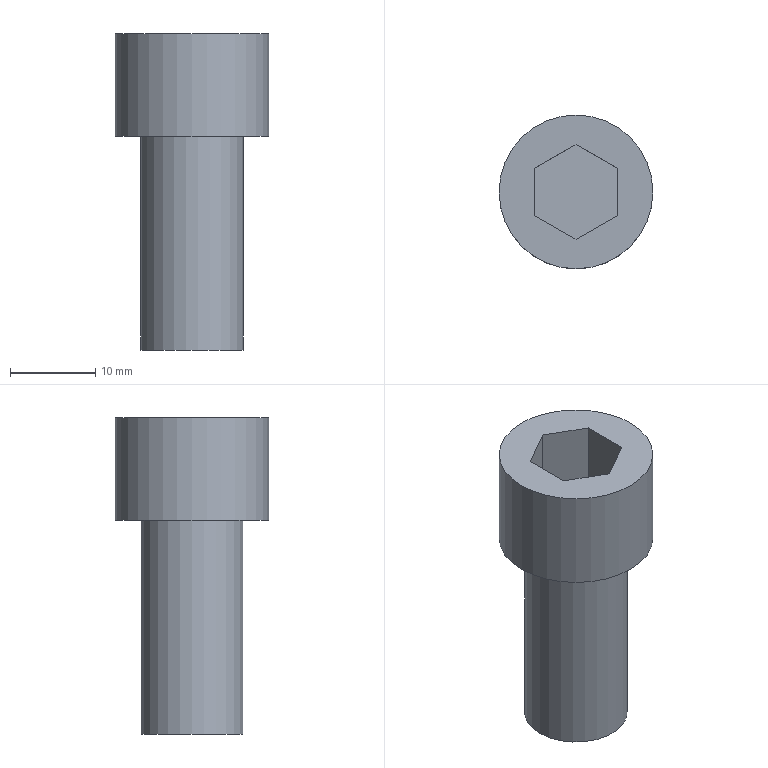Part | NX | features solid 2 | 1 solid | 12 faces | box 18 x 18 x 37 mm | volume 5306 mm3 | plane 10 | cylinder 2 | commonest cylinder face diameters 12 x1 18 x1
STEP:
#1=CARTESIAN_POINT('',(665.2,72.229,-53.));
#2=VERTEX_POINT('',#1);
#3=CARTESIAN_POINT('',(670.,69.457,-53.));
#4=VERTEX_POINT('',#3);
#5=CARTESIAN_POINT('',(667.6,70.843,-53.));
#6=DIRECTION('',(0.866,-0.5,0.));
#7=VECTOR('',#6,1000.);
#8=LINE('',#5,#7);
#9=EDGE_CURVE('',#2,#4,#8,.T.);
#10=ORIENTED_EDGE('',*,*,#9,.F.);
#11=CARTESIAN_POINT('',(665.2,77.771,-53.));
#12=VERTEX_POINT('',#11);
#13=CARTESIAN_POINT('',(665.2,75.,-53.));
#14=DIRECTION('',(0.,-1.,0.));
#15=VECTOR('',#14,1000.);
#16=LINE('',#13,#15);
#17=EDGE_CURVE('',#12,#2,#16,.T.);
#18=ORIENTED_EDGE('',*,*,#17,.F.);
#19=CARTESIAN_POINT('',(670.,80.543,-53.));
#20=VERTEX_POINT('',#19);
#21=CARTESIAN_POINT('',(667.6,79.157,-53.));
#22=DIRECTION('',(-0.866,-0.5,0.));
#23=VECTOR('',#22,1000.);
#24=LINE('',#21,#23);
#25=EDGE_CURVE('',#20,#12,#24,.T.);
#26=ORIENTED_EDGE('',*,*,#25,.F.);
#27=CARTESIAN_POINT('',(674.8,77.771,-53.));
#28=VERTEX_POINT('',#27);
#29=CARTESIAN_POINT('',(672.4,79.157,-53.));
#30=DIRECTION('',(-0.866,0.5,0.));
#31=VECTOR('',#30,1000.);
#32=LINE('',#29,#31);
#33=EDGE_CURVE('',#28,#20,#32,.T.);
#34=ORIENTED_EDGE('',*,*,#33,.F.);
#35=CARTESIAN_POINT('',(674.8,72.229,-53.));
#36=VERTEX_POINT('',#35);
#37=CARTESIAN_POINT('',(674.8,75.,-53.));
#38=DIRECTION('',(0.,1.,0.));
#39=VECTOR('',#38,1000.);
#40=LINE('',#37,#39);
#41=EDGE_CURVE('',#36,#28,#40,.T.);
#42=ORIENTED_EDGE('',*,*,#41,.F.);
#43=CARTESIAN_POINT('',(672.4,70.843,-53.));
#44=DIRECTION('',(0.866,0.5,0.));
#45=VECTOR('',#44,1000.);
#46=LINE('',#43,#45);
#47=EDGE_CURVE('',#4,#36,#46,.T.);
#48=ORIENTED_EDGE('',*,*,#47,.F.);
#49=EDGE_LOOP('',(#10,#18,#26,#34,#42,#48));
#50=FACE_BOUND('',#49,.T.);
#51=CARTESIAN_POINT('',(661.,75.,-53.));
#52=VERTEX_POINT('',#51);
#53=CARTESIAN_POINT('',(670.,75.,-53.));
#54=DIRECTION('',(0.,0.,-1.));
#55=DIRECTION('',(-1.,0.,0.));
#56=AXIS2_PLACEMENT_3D('',#53,#54,#55);
#57=CIRCLE('',#56,9.);
#58=EDGE_CURVE('',#52,#52,#57,.T.);
#59=ORIENTED_EDGE('',*,*,#58,.F.);
#60=EDGE_LOOP('',(#59));
#61=FACE_BOUND('',#60,.T.);
#62=CARTESIAN_POINT('',(670.,75.,-53.));
#63=DIRECTION('',(0.,0.,1.));
#64=DIRECTION('',(1.,0.,0.));
#65=AXIS2_PLACEMENT_3D('',#62,#63,#64);
#66=PLANE('',#65);
#67=ADVANCED_FACE('',(#50,#61),#66,.T.);
#68=CARTESIAN_POINT('',(664.,75.,-65.));
#69=VERTEX_POINT('',#68);
#70=CARTESIAN_POINT('',(670.,75.,-65.));
#71=DIRECTION('',(0.,0.,-1.));
#72=DIRECTION('',(-1.,0.,0.));
#73=AXIS2_PLACEMENT_3D('',#70,#71,#72);
#74=CIRCLE('',#73,6.);
#75=EDGE_CURVE('',#69,#69,#74,.T.);
#76=ORIENTED_EDGE('',*,*,#75,.F.);
#77=EDGE_LOOP('',(#76));
#78=FACE_BOUND('',#77,.T.);
#79=CARTESIAN_POINT('',(679.,75.,-65.));
#80=VERTEX_POINT('',#79);
#81=CARTESIAN_POINT('',(670.,75.,-65.));
#82=DIRECTION('',(0.,0.,1.));
#83=DIRECTION('',(1.,0.,0.));
#84=AXIS2_PLACEMENT_3D('',#81,#82,#83);
#85=CIRCLE('',#84,9.);
#86=EDGE_CURVE('',#80,#80,#85,.T.);
#87=ORIENTED_EDGE('',*,*,#86,.F.);
#88=EDGE_LOOP('',(#87));
#89=FACE_BOUND('',#88,.T.);
#90=CARTESIAN_POINT('',(670.,75.,-65.));
#91=DIRECTION('',(0.,0.,-1.));
#92=DIRECTION('',(-1.,0.,0.));
#93=AXIS2_PLACEMENT_3D('',#90,#91,#92);
#94=PLANE('',#93);
#95=ADVANCED_FACE('',(#78,#89),#94,.T.);
#96=ORIENTED_EDGE('',*,*,#58,.T.);
#97=EDGE_LOOP('',(#96));
#98=FACE_BOUND('',#97,.T.);
#99=ORIENTED_EDGE('',*,*,#86,.T.);
#100=EDGE_LOOP('',(#99));
#101=FACE_BOUND('',#100,.T.);
#102=CARTESIAN_POINT('',(670.,75.,-65.));
#103=DIRECTION('',(0.,0.,1.));
#104=DIRECTION('',(1.,0.,0.));
#105=AXIS2_PLACEMENT_3D('',#102,#103,#104);
#106=CYLINDRICAL_SURFACE('',#105,9.);
#107=ADVANCED_FACE('',(#98,#101),#106,.T.);
#108=ORIENTED_EDGE('',*,*,#9,.T.);
#109=CARTESIAN_POINT('',(670.,69.457,-60.2));
#110=VERTEX_POINT('',#109);
#111=CARTESIAN_POINT('',(670.,69.457,-60.2));
#112=DIRECTION('',(0.,0.,1.));
#113=VECTOR('',#112,1000.);
#114=LINE('',#111,#113);
#115=EDGE_CURVE('',#110,#4,#114,.T.);
#116=ORIENTED_EDGE('',*,*,#115,.F.);
#117=CARTESIAN_POINT('',(665.2,72.229,-60.2));
#118=VERTEX_POINT('',#117);
#119=CARTESIAN_POINT('',(665.2,72.229,-60.2));
#120=DIRECTION('',(0.866,-0.5,0.));
#121=VECTOR('',#120,1000.);
#122=LINE('',#119,#121);
#123=EDGE_CURVE('',#118,#110,#122,.T.);
#124=ORIENTED_EDGE('',*,*,#123,.F.);
#125=CARTESIAN_POINT('',(665.2,72.229,-60.2));
#126=DIRECTION('',(0.,0.,1.));
#127=VECTOR('',#126,1000.);
#128=LINE('',#125,#127);
#129=EDGE_CURVE('',#118,#2,#128,.T.);
#130=ORIENTED_EDGE('',*,*,#129,.T.);
#131=EDGE_LOOP('',(#108,#116,#124,#130));
#132=FACE_BOUND('',#131,.T.);
#133=CARTESIAN_POINT('',(667.6,70.843,-54.2));
#134=DIRECTION('',(-0.5,-0.866,0.));
#135=DIRECTION('',(0.866,-0.5,0.));
#136=AXIS2_PLACEMENT_3D('',#133,#134,#135);
#137=PLANE('',#136);
#138=ADVANCED_FACE('',(#132),#137,.F.);
#139=ORIENTED_EDGE('',*,*,#17,.T.);
#140=ORIENTED_EDGE('',*,*,#129,.F.);
#141=CARTESIAN_POINT('',(665.2,77.771,-60.2));
#142=VERTEX_POINT('',#141);
#143=CARTESIAN_POINT('',(665.2,77.771,-60.2));
#144=DIRECTION('',(0.,-1.,0.));
#145=VECTOR('',#144,1000.);
#146=LINE('',#143,#145);
#147=EDGE_CURVE('',#142,#118,#146,.T.);
#148=ORIENTED_EDGE('',*,*,#147,.F.);
#149=CARTESIAN_POINT('',(665.2,77.771,-60.2));
#150=DIRECTION('',(0.,0.,1.));
#151=VECTOR('',#150,1000.);
#152=LINE('',#149,#151);
#153=EDGE_CURVE('',#142,#12,#152,.T.);
#154=ORIENTED_EDGE('',*,*,#153,.T.);
#155=EDGE_LOOP('',(#139,#140,#148,#154));
#156=FACE_BOUND('',#155,.T.);
#157=CARTESIAN_POINT('',(665.2,75.,-54.2));
#158=DIRECTION('',(-1.,0.,0.));
#159=DIRECTION('',(0.,0.,1.));
#160=AXIS2_PLACEMENT_3D('',#157,#158,#159);
#161=PLANE('',#160);
#162=ADVANCED_FACE('',(#156),#161,.F.);
#163=ORIENTED_EDGE('',*,*,#25,.T.);
#164=ORIENTED_EDGE('',*,*,#153,.F.);
#165=CARTESIAN_POINT('',(670.,80.543,-60.2));
#166=VERTEX_POINT('',#165);
#167=CARTESIAN_POINT('',(670.,80.543,-60.2));
#168=DIRECTION('',(-0.866,-0.5,0.));
#169=VECTOR('',#168,1000.);
#170=LINE('',#167,#169);
#171=EDGE_CURVE('',#166,#142,#170,.T.);
#172=ORIENTED_EDGE('',*,*,#171,.F.);
#173=CARTESIAN_POINT('',(670.,80.543,-60.2));
#174=DIRECTION('',(0.,0.,1.));
#175=VECTOR('',#174,1000.);
#176=LINE('',#173,#175);
#177=EDGE_CURVE('',#166,#20,#176,.T.);
#178=ORIENTED_EDGE('',*,*,#177,.T.);
#179=EDGE_LOOP('',(#163,#164,#172,#178));
#180=FACE_BOUND('',#179,.T.);
#181=CARTESIAN_POINT('',(667.6,79.157,-54.2));
#182=DIRECTION('',(-0.5,0.866,0.));
#183=DIRECTION('',(-0.866,-0.5,0.));
#184=AXIS2_PLACEMENT_3D('',#181,#182,#183);
#185=PLANE('',#184);
#186=ADVANCED_FACE('',(#180),#185,.F.);
#187=ORIENTED_EDGE('',*,*,#33,.T.);
#188=ORIENTED_EDGE('',*,*,#177,.F.);
#189=CARTESIAN_POINT('',(674.8,77.771,-60.2));
#190=VERTEX_POINT('',#189);
#191=CARTESIAN_POINT('',(674.8,77.771,-60.2));
#192=DIRECTION('',(-0.866,0.5,0.));
#193=VECTOR('',#192,1000.);
#194=LINE('',#191,#193);
#195=EDGE_CURVE('',#190,#166,#194,.T.);
#196=ORIENTED_EDGE('',*,*,#195,.F.);
#197=CARTESIAN_POINT('',(674.8,77.771,-60.2));
#198=DIRECTION('',(0.,0.,1.));
#199=VECTOR('',#198,1000.);
#200=LINE('',#197,#199);
#201=EDGE_CURVE('',#190,#28,#200,.T.);
#202=ORIENTED_EDGE('',*,*,#201,.T.);
#203=EDGE_LOOP('',(#187,#188,#196,#202));
#204=FACE_BOUND('',#203,.T.);
#205=CARTESIAN_POINT('',(672.4,79.157,-54.2));
#206=DIRECTION('',(0.5,0.866,0.));
#207=DIRECTION('',(-0.866,0.5,0.));
#208=AXIS2_PLACEMENT_3D('',#205,#206,#207);
#209=PLANE('',#208);
#210=ADVANCED_FACE('',(#204),#209,.F.);
#211=ORIENTED_EDGE('',*,*,#41,.T.);
#212=ORIENTED_EDGE('',*,*,#201,.F.);
#213=CARTESIAN_POINT('',(674.8,72.229,-60.2));
#214=VERTEX_POINT('',#213);
#215=CARTESIAN_POINT('',(674.8,72.229,-60.2));
#216=DIRECTION('',(0.,1.,0.));
#217=VECTOR('',#216,1000.);
#218=LINE('',#215,#217);
#219=EDGE_CURVE('',#214,#190,#218,.T.);
#220=ORIENTED_EDGE('',*,*,#219,.F.);
#221=CARTESIAN_POINT('',(674.8,72.229,-60.2));
#222=DIRECTION('',(0.,0.,1.));
#223=VECTOR('',#222,1000.);
#224=LINE('',#221,#223);
#225=EDGE_CURVE('',#214,#36,#224,.T.);
#226=ORIENTED_EDGE('',*,*,#225,.T.);
#227=EDGE_LOOP('',(#211,#212,#220,#226));
#228=FACE_BOUND('',#227,.T.);
#229=CARTESIAN_POINT('',(674.8,75.,-54.2));
#230=DIRECTION('',(1.,0.,0.));
#231=DIRECTION('',(0.,0.,-1.));
#232=AXIS2_PLACEMENT_3D('',#229,#230,#231);
#233=PLANE('',#232);
#234=ADVANCED_FACE('',(#228),#233,.F.);
#235=ORIENTED_EDGE('',*,*,#47,.T.);
#236=ORIENTED_EDGE('',*,*,#225,.F.);
#237=CARTESIAN_POINT('',(670.,69.457,-60.2));
#238=DIRECTION('',(0.866,0.5,0.));
#239=VECTOR('',#238,1000.);
#240=LINE('',#237,#239);
#241=EDGE_CURVE('',#110,#214,#240,.T.);
#242=ORIENTED_EDGE('',*,*,#241,.F.);
#243=ORIENTED_EDGE('',*,*,#115,.T.);
#244=EDGE_LOOP('',(#235,#236,#242,#243));
#245=FACE_BOUND('',#244,.T.);
#246=CARTESIAN_POINT('',(672.4,70.843,-54.2));
#247=DIRECTION('',(0.5,-0.866,0.));
#248=DIRECTION('',(0.866,0.5,0.));
#249=AXIS2_PLACEMENT_3D('',#246,#247,#248);
#250=PLANE('',#249);
#251=ADVANCED_FACE('',(#245),#250,.F.);
#252=ORIENTED_EDGE('',*,*,#241,.T.);
#253=ORIENTED_EDGE('',*,*,#219,.T.);
#254=ORIENTED_EDGE('',*,*,#195,.T.);
#255=ORIENTED_EDGE('',*,*,#171,.T.);
#256=ORIENTED_EDGE('',*,*,#147,.T.);
#257=ORIENTED_EDGE('',*,*,#123,.T.);
#258=EDGE_LOOP('',(#252,#253,#254,#255,#256,#257));
#259=FACE_BOUND('',#258,.T.);
#260=CARTESIAN_POINT('',(670.,75.,-60.2));
#261=DIRECTION('',(0.,0.,-1.));
#262=DIRECTION('',(-1.,0.,0.));
#263=AXIS2_PLACEMENT_3D('',#260,#261,#262);
#264=PLANE('',#263);
#265=ADVANCED_FACE('',(#259),#264,.F.);
#266=CARTESIAN_POINT('',(676.,75.,-90.));
#267=VERTEX_POINT('',#266);
#268=CARTESIAN_POINT('',(670.,75.,-90.));
#269=DIRECTION('',(0.,0.,1.));
#270=DIRECTION('',(1.,0.,0.));
#271=AXIS2_PLACEMENT_3D('',#268,#269,#270);
#272=CIRCLE('',#271,6.);
#273=EDGE_CURVE('',#267,#267,#272,.T.);
#274=ORIENTED_EDGE('',*,*,#273,.F.);
#275=EDGE_LOOP('',(#274));
#276=FACE_BOUND('',#275,.T.);
#277=CARTESIAN_POINT('',(670.,75.,-90.));
#278=DIRECTION('',(0.,0.,-1.));
#279=DIRECTION('',(-1.,0.,0.));
#280=AXIS2_PLACEMENT_3D('',#277,#278,#279);
#281=PLANE('',#280);
#282=ADVANCED_FACE('',(#276),#281,.T.);
#283=ORIENTED_EDGE('',*,*,#273,.T.);
#284=EDGE_LOOP('',(#283));
#285=FACE_BOUND('',#284,.T.);
#286=ORIENTED_EDGE('',*,*,#75,.T.);
#287=EDGE_LOOP('',(#286));
#288=FACE_BOUND('',#287,.T.);
#289=CARTESIAN_POINT('',(670.,75.,-65.));
#290=DIRECTION('',(0.,0.,-1.));
#291=DIRECTION('',(-1.,0.,0.));
#292=AXIS2_PLACEMENT_3D('',#289,#290,#291);
#293=CYLINDRICAL_SURFACE('',#292,6.);
#294=ADVANCED_FACE('',(#285,#288),#293,.T.);
#295=CLOSED_SHELL('',(#67,#95,#107,#138,#162,#186,#210,#234,#251,#265,#282,#294));
#296=MANIFOLD_SOLID_BREP('',#295);
#297=(LENGTH_UNIT()NAMED_UNIT(*)SI_UNIT(.MILLI.,.METRE.));
#298=UNCERTAINTY_MEASURE_WITH_UNIT(LENGTH_MEASURE(0.00001),#297,'','');
#299=(NAMED_UNIT(*)PLANE_ANGLE_UNIT()SI_UNIT($,.RADIAN.));
#300=(NAMED_UNIT(*)SI_UNIT($,.STERADIAN.)SOLID_ANGLE_UNIT());
#301=(GEOMETRIC_REPRESENTATION_CONTEXT(3)GLOBAL_UNCERTAINTY_ASSIGNED_CONTEXT((#298))GLOBAL_UNIT_ASSIGNED_CONTEXT((#297,#299,#300))REPRESENTATION_CONTEXT('',''));
#302=ADVANCED_BREP_SHAPE_REPRESENTATION('',(#296),#301);